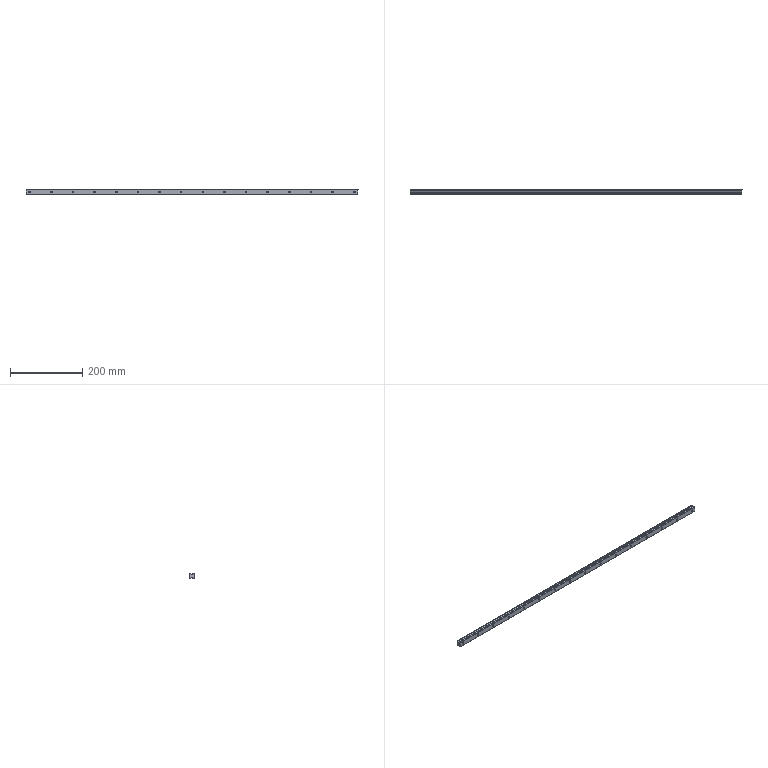Part | SolidWorks | features BaseBody 1 | 1 solid | 105 faces | box 920 x 12.53 x 15 mm | volume 149023 mm3 | cylinder 71 | plane 34 | commonest cylinder face diameters 4.5 x32 8 x32 2.9 x4 1.4 x3